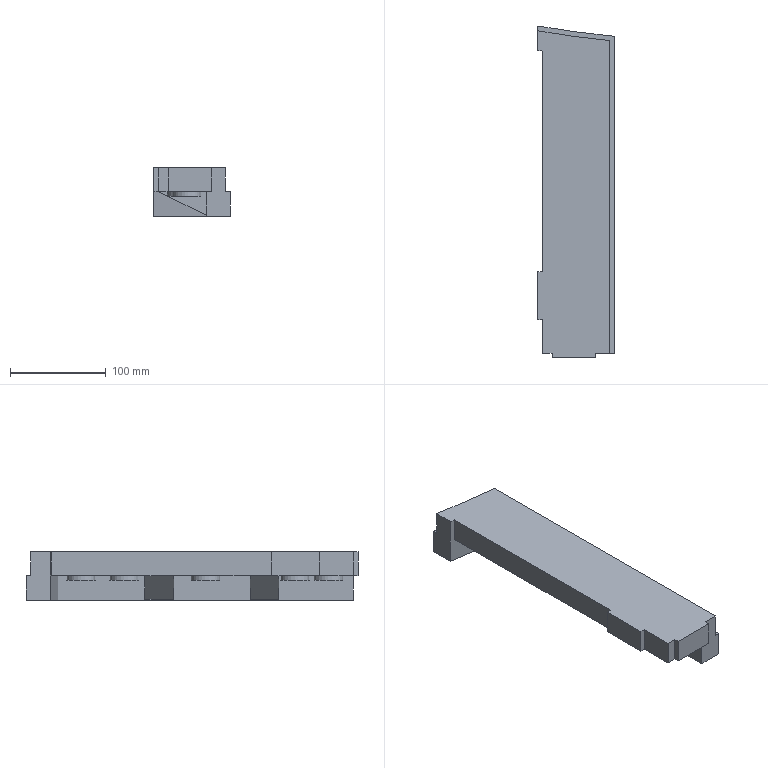Part | NX | features solid 2 | 1 solid | 39 faces | box 80 x 346.995 x 51 mm | volume 901163 mm3 | plane 31 | cylinder 5 | spline 3 | commonest cylinder face diameters 30 x5
STEP:
#1=CARTESIAN_POINT('',(-400.,-480.,45.));
#2=VERTEX_POINT('',#1);
#3=CARTESIAN_POINT('',(-400.,-249.179,45.));
#4=VERTEX_POINT('',#3);
#5=CARTESIAN_POINT('',(-400.,-330.218,45.));
#6=DIRECTION('',(0.,1.,0.));
#7=VECTOR('',#6,1000.);
#8=LINE('',#5,#7);
#9=EDGE_CURVE('',#2,#4,#8,.T.);
#10=ORIENTED_EDGE('',*,*,#9,.T.);
#11=CARTESIAN_POINT('',(-400.,-249.179,20.));
#12=VERTEX_POINT('',#11);
#13=CARTESIAN_POINT('',(-400.,-249.179,45.));
#14=DIRECTION('',(0.,0.,-1.));
#15=VECTOR('',#14,1000.);
#16=LINE('',#13,#15);
#17=EDGE_CURVE('',#4,#12,#16,.T.);
#18=ORIENTED_EDGE('',*,*,#17,.T.);
#19=CARTESIAN_POINT('',(-400.,-347.246,20.));
#20=VERTEX_POINT('',#19);
#21=CARTESIAN_POINT('',(-400.,-330.218,20.));
#22=DIRECTION('',(0.,1.,0.));
#23=VECTOR('',#22,1000.);
#24=LINE('',#21,#23);
#25=EDGE_CURVE('',#20,#12,#24,.T.);
#26=ORIENTED_EDGE('',*,*,#25,.F.);
#27=CARTESIAN_POINT('',(-400.,-377.246,20.));
#28=VERTEX_POINT('',#27);
#29=CARTESIAN_POINT('',(-400.,-347.246,20.));
#30=DIRECTION('',(0.,-1.,0.));
#31=VECTOR('',#30,1000.);
#32=LINE('',#29,#31);
#33=EDGE_CURVE('',#20,#28,#32,.T.);
#34=ORIENTED_EDGE('',*,*,#33,.T.);
#35=CARTESIAN_POINT('',(-400.,-457.246,20.));
#36=VERTEX_POINT('',#35);
#37=CARTESIAN_POINT('',(-400.,-330.218,20.));
#38=DIRECTION('',(0.,1.,0.));
#39=VECTOR('',#38,1000.);
#40=LINE('',#37,#39);
#41=EDGE_CURVE('',#36,#28,#40,.T.);
#42=ORIENTED_EDGE('',*,*,#41,.F.);
#43=CARTESIAN_POINT('',(-400.,-480.,20.));
#44=VERTEX_POINT('',#43);
#45=CARTESIAN_POINT('',(-400.,-457.246,20.));
#46=DIRECTION('',(0.,-1.,0.));
#47=VECTOR('',#46,1000.);
#48=LINE('',#45,#47);
#49=EDGE_CURVE('',#36,#44,#48,.T.);
#50=ORIENTED_EDGE('',*,*,#49,.T.);
#51=CARTESIAN_POINT('',(-400.,-480.,20.));
#52=DIRECTION('',(0.,0.,-1.));
#53=VECTOR('',#52,1000.);
#54=LINE('',#51,#53);
#55=EDGE_CURVE('',#44,#2,#54,.F.);
#56=ORIENTED_EDGE('',*,*,#55,.T.);
#57=EDGE_LOOP('',(#10,#18,#26,#34,#42,#50,#56));
#58=FACE_BOUND('',#57,.T.);
#59=CARTESIAN_POINT('',(-400.,-330.218,45.));
#60=DIRECTION('',(-1.,0.,0.));
#61=DIRECTION('',(0.,0.,1.));
#62=AXIS2_PLACEMENT_3D('',#59,#60,#61);
#63=PLANE('',#62);
#64=ADVANCED_FACE('',(#58),#63,.T.);
#65=CARTESIAN_POINT('',(-350.,-256.193,20.));
#66=VERTEX_POINT('',#65);
#67=CARTESIAN_POINT('',(-350.,-347.246,20.));
#68=VERTEX_POINT('',#67);
#69=CARTESIAN_POINT('',(-350.,-401.561,20.));
#70=DIRECTION('',(0.,1.,0.));
#71=VECTOR('',#70,1000.);
#72=LINE('',#69,#71);
#73=EDGE_CURVE('',#66,#68,#72,.F.);
#74=ORIENTED_EDGE('',*,*,#73,.F.);
#75=CARTESIAN_POINT('',(-350.,-256.193,-6.));
#76=VERTEX_POINT('',#75);
#77=CARTESIAN_POINT('',(-350.,-256.193,45.));
#78=DIRECTION('',(0.,0.,-1.));
#79=VECTOR('',#78,1000.);
#80=LINE('',#77,#79);
#81=EDGE_CURVE('',#66,#76,#80,.T.);
#82=ORIENTED_EDGE('',*,*,#81,.T.);
#83=CARTESIAN_POINT('',(-350.,-565.,-6.));
#84=VERTEX_POINT('',#83);
#85=CARTESIAN_POINT('',(-350.,-1052.635,-6.));
#86=DIRECTION('',(0.,-1.,0.));
#87=VECTOR('',#86,1000.);
#88=LINE('',#85,#87);
#89=EDGE_CURVE('',#84,#76,#88,.F.);
#90=ORIENTED_EDGE('',*,*,#89,.F.);
#91=CARTESIAN_POINT('',(-350.,-565.,20.));
#92=VERTEX_POINT('',#91);
#93=CARTESIAN_POINT('',(-350.,-565.,25.));
#94=DIRECTION('',(0.,0.,1.));
#95=VECTOR('',#94,1000.);
#96=LINE('',#93,#95);
#97=EDGE_CURVE('',#92,#84,#96,.F.);
#98=ORIENTED_EDGE('',*,*,#97,.F.);
#99=CARTESIAN_POINT('',(-350.,-487.246,20.));
#100=VERTEX_POINT('',#99);
#101=CARTESIAN_POINT('',(-350.,-401.561,20.));
#102=DIRECTION('',(0.,1.,0.));
#103=VECTOR('',#102,1000.);
#104=LINE('',#101,#103);
#105=EDGE_CURVE('',#100,#92,#104,.F.);
#106=ORIENTED_EDGE('',*,*,#105,.F.);
#107=CARTESIAN_POINT('',(-350.,-487.246,-5.));
#108=VERTEX_POINT('',#107);
#109=CARTESIAN_POINT('',(-350.,-487.246,20.));
#110=DIRECTION('',(0.,0.,-1.));
#111=VECTOR('',#110,1000.);
#112=LINE('',#109,#111);
#113=EDGE_CURVE('',#100,#108,#112,.T.);
#114=ORIENTED_EDGE('',*,*,#113,.T.);
#115=CARTESIAN_POINT('',(-350.,-457.246,-5.));
#116=VERTEX_POINT('',#115);
#117=CARTESIAN_POINT('',(-350.,-457.246,-5.));
#118=DIRECTION('',(0.,1.,0.));
#119=VECTOR('',#118,1000.);
#120=LINE('',#117,#119);
#121=EDGE_CURVE('',#116,#108,#120,.F.);
#122=ORIENTED_EDGE('',*,*,#121,.F.);
#123=CARTESIAN_POINT('',(-350.,-457.246,20.));
#124=VERTEX_POINT('',#123);
#125=CARTESIAN_POINT('',(-350.,-457.246,20.));
#126=DIRECTION('',(0.,0.,-1.));
#127=VECTOR('',#126,1000.);
#128=LINE('',#125,#127);
#129=EDGE_CURVE('',#124,#116,#128,.T.);
#130=ORIENTED_EDGE('',*,*,#129,.F.);
#131=CARTESIAN_POINT('',(-350.,-377.246,20.));
#132=VERTEX_POINT('',#131);
#133=CARTESIAN_POINT('',(-350.,-401.561,20.));
#134=DIRECTION('',(0.,1.,0.));
#135=VECTOR('',#134,1000.);
#136=LINE('',#133,#135);
#137=EDGE_CURVE('',#132,#124,#136,.F.);
#138=ORIENTED_EDGE('',*,*,#137,.F.);
#139=CARTESIAN_POINT('',(-350.,-377.246,-5.));
#140=VERTEX_POINT('',#139);
#141=CARTESIAN_POINT('',(-350.,-377.246,20.));
#142=DIRECTION('',(0.,0.,-1.));
#143=VECTOR('',#142,1000.);
#144=LINE('',#141,#143);
#145=EDGE_CURVE('',#132,#140,#144,.T.);
#146=ORIENTED_EDGE('',*,*,#145,.T.);
#147=CARTESIAN_POINT('',(-350.,-347.246,-5.));
#148=VERTEX_POINT('',#147);
#149=CARTESIAN_POINT('',(-350.,-347.246,-5.));
#150=DIRECTION('',(0.,1.,0.));
#151=VECTOR('',#150,1000.);
#152=LINE('',#149,#151);
#153=EDGE_CURVE('',#148,#140,#152,.F.);
#154=ORIENTED_EDGE('',*,*,#153,.F.);
#155=CARTESIAN_POINT('',(-350.,-347.246,20.));
#156=DIRECTION('',(0.,0.,-1.));
#157=VECTOR('',#156,1000.);
#158=LINE('',#155,#157);
#159=EDGE_CURVE('',#68,#148,#158,.T.);
#160=ORIENTED_EDGE('',*,*,#159,.F.);
#161=EDGE_LOOP('',(#74,#82,#90,#98,#106,#114,#122,#130,#138,#146,#154,#160));
#162=FACE_BOUND('',#161,.T.);
#163=CARTESIAN_POINT('',(-350.,-560.,25.));
#164=DIRECTION('',(-1.,0.,0.));
#165=DIRECTION('',(0.,0.,1.));
#166=AXIS2_PLACEMENT_3D('',#163,#164,#165);
#167=PLANE('',#166);
#168=ADVANCED_FACE('',(#162),#167,.T.);
#169=CARTESIAN_POINT('',(-390.,-565.,20.));
#170=VERTEX_POINT('',#169);
#171=CARTESIAN_POINT('',(-400.,-565.,20.));
#172=VERTEX_POINT('',#171);
#173=CARTESIAN_POINT('',(-53.05,-565.,20.));
#174=DIRECTION('',(-1.,0.,0.));
#175=VECTOR('',#174,1000.);
#176=LINE('',#173,#175);
#177=EDGE_CURVE('',#170,#172,#176,.T.);
#178=ORIENTED_EDGE('',*,*,#177,.F.);
#179=CARTESIAN_POINT('',(-390.,-565.,45.));
#180=VERTEX_POINT('',#179);
#181=CARTESIAN_POINT('',(-390.,-565.,25.));
#182=DIRECTION('',(0.,0.,-1.));
#183=VECTOR('',#182,1000.);
#184=LINE('',#181,#183);
#185=EDGE_CURVE('',#170,#180,#184,.F.);
#186=ORIENTED_EDGE('',*,*,#185,.T.);
#187=CARTESIAN_POINT('',(-400.,-565.,45.));
#188=VERTEX_POINT('',#187);
#189=CARTESIAN_POINT('',(-582.311,-565.,45.));
#190=DIRECTION('',(1.,0.,0.));
#191=VECTOR('',#190,1000.);
#192=LINE('',#189,#191);
#193=EDGE_CURVE('',#180,#188,#192,.F.);
#194=ORIENTED_EDGE('',*,*,#193,.T.);
#195=CARTESIAN_POINT('',(-400.,-565.,25.));
#196=DIRECTION('',(0.,0.,-1.));
#197=VECTOR('',#196,1000.);
#198=LINE('',#195,#197);
#199=EDGE_CURVE('',#172,#188,#198,.F.);
#200=ORIENTED_EDGE('',*,*,#199,.F.);
#201=EDGE_LOOP('',(#178,#186,#194,#200));
#202=FACE_BOUND('',#201,.T.);
#203=CARTESIAN_POINT('',(-325.,-565.,25.));
#204=DIRECTION('',(0.,-1.,0.));
#205=DIRECTION('',(0.,0.,-1.));
#206=AXIS2_PLACEMENT_3D('',#203,#204,#205);
#207=PLANE('',#206);
#208=ADVANCED_FACE('',(#202),#207,.T.);
#209=ORIENTED_EDGE('',*,*,#25,.T.);
#210=CARTESIAN_POINT('',(-405.,-248.354,20.));
#211=CARTESIAN_POINT('',(-398.879,-249.375,20.));
#212=CARTESIAN_POINT('',(-378.346,-252.669,20.));
#213=CARTESIAN_POINT('',(-351.447,-256.141,20.));
#214=CARTESIAN_POINT('',(-331.018,-258.325,20.));
#215=CARTESIAN_POINT('',(-325.,-258.957,20.));
#216=B_SPLINE_CURVE_WITH_KNOTS('',3,(#210,#211,#212,#213,#214,#215),.UNSPECIFIED.,.F.,.F.,(4,1,1,4),(0.,0.231,0.7722,1.),.UNSPECIFIED.);
#217=EDGE_CURVE('',#12,#66,#216,.T.);
#218=ORIENTED_EDGE('',*,*,#217,.T.);
#219=ORIENTED_EDGE('',*,*,#73,.T.);
#220=CARTESIAN_POINT('',(-350.,-347.246,20.));
#221=DIRECTION('',(-1.,0.,0.));
#222=VECTOR('',#221,1000.);
#223=LINE('',#220,#222);
#224=EDGE_CURVE('',#68,#20,#223,.T.);
#225=ORIENTED_EDGE('',*,*,#224,.T.);
#226=EDGE_LOOP('',(#209,#218,#219,#225));
#227=FACE_BOUND('',#226,.T.);
#228=CARTESIAN_POINT('',(-390.611,-325.558,20.));
#229=VERTEX_POINT('',#228);
#230=CARTESIAN_POINT('',(-375.611,-325.558,20.));
#231=DIRECTION('',(0.,0.,-1.));
#232=DIRECTION('',(-1.,0.,0.));
#233=AXIS2_PLACEMENT_3D('',#230,#231,#232);
#234=CIRCLE('',#233,15.);
#235=EDGE_CURVE('',#229,#229,#234,.T.);
#236=ORIENTED_EDGE('',*,*,#235,.F.);
#237=EDGE_LOOP('',(#236));
#238=FACE_BOUND('',#237,.T.);
#239=CARTESIAN_POINT('',(-385.611,-280.558,20.));
#240=VERTEX_POINT('',#239);
#241=CARTESIAN_POINT('',(-370.611,-280.558,20.));
#242=DIRECTION('',(0.,0.,-1.));
#243=DIRECTION('',(-1.,0.,0.));
#244=AXIS2_PLACEMENT_3D('',#241,#242,#243);
#245=CIRCLE('',#244,15.);
#246=EDGE_CURVE('',#240,#240,#245,.T.);
#247=ORIENTED_EDGE('',*,*,#246,.F.);
#248=EDGE_LOOP('',(#247));
#249=FACE_BOUND('',#248,.T.);
#250=CARTESIAN_POINT('',(-53.05,-401.561,20.));
#251=DIRECTION('',(0.,0.,-1.));
#252=DIRECTION('',(-1.,0.,0.));
#253=AXIS2_PLACEMENT_3D('',#250,#251,#252);
#254=PLANE('',#253);
#255=ADVANCED_FACE('',(#227,#238,#249),#254,.T.);
#256=CARTESIAN_POINT('',(-390.611,-410.558,20.));
#257=VERTEX_POINT('',#256);
#258=CARTESIAN_POINT('',(-375.611,-410.558,20.));
#259=DIRECTION('',(0.,0.,-1.));
#260=DIRECTION('',(-1.,0.,0.));
#261=AXIS2_PLACEMENT_3D('',#258,#259,#260);
#262=CIRCLE('',#261,15.);
#263=EDGE_CURVE('',#257,#257,#262,.T.);
#264=ORIENTED_EDGE('',*,*,#263,.F.);
#265=EDGE_LOOP('',(#264));
#266=FACE_BOUND('',#265,.T.);
#267=ORIENTED_EDGE('',*,*,#137,.T.);
#268=CARTESIAN_POINT('',(-350.,-457.246,20.));
#269=DIRECTION('',(-1.,0.,0.));
#270=VECTOR('',#269,1000.);
#271=LINE('',#268,#270);
#272=EDGE_CURVE('',#124,#36,#271,.T.);
#273=ORIENTED_EDGE('',*,*,#272,.T.);
#274=ORIENTED_EDGE('',*,*,#41,.T.);
#275=CARTESIAN_POINT('',(-350.,-377.246,20.));
#276=DIRECTION('',(-1.,0.,0.));
#277=VECTOR('',#276,1000.);
#278=LINE('',#275,#277);
#279=EDGE_CURVE('',#132,#28,#278,.T.);
#280=ORIENTED_EDGE('',*,*,#279,.F.);
#281=EDGE_LOOP('',(#267,#273,#274,#280));
#282=FACE_BOUND('',#281,.T.);
#283=CARTESIAN_POINT('',(-53.05,-401.561,20.));
#284=DIRECTION('',(0.,0.,-1.));
#285=DIRECTION('',(-1.,0.,0.));
#286=AXIS2_PLACEMENT_3D('',#283,#284,#285);
#287=PLANE('',#286);
#288=ADVANCED_FACE('',(#266,#282),#287,.T.);
#289=CARTESIAN_POINT('',(-390.611,-503.935,20.));
#290=VERTEX_POINT('',#289);
#291=CARTESIAN_POINT('',(-375.611,-503.935,20.));
#292=DIRECTION('',(0.,0.,-1.));
#293=DIRECTION('',(-1.,0.,0.));
#294=AXIS2_PLACEMENT_3D('',#291,#292,#293);
#295=CIRCLE('',#294,15.);
#296=EDGE_CURVE('',#290,#290,#295,.T.);
#297=ORIENTED_EDGE('',*,*,#296,.F.);
#298=EDGE_LOOP('',(#297));
#299=FACE_BOUND('',#298,.T.);
#300=CARTESIAN_POINT('',(-400.,-530.,20.));
#301=VERTEX_POINT('',#300);
#302=CARTESIAN_POINT('',(-400.,-330.218,20.));
#303=DIRECTION('',(0.,1.,0.));
#304=VECTOR('',#303,1000.);
#305=LINE('',#302,#304);
#306=EDGE_CURVE('',#172,#301,#305,.T.);
#307=ORIENTED_EDGE('',*,*,#306,.T.);
#308=CARTESIAN_POINT('',(-405.,-530.,20.));
#309=VERTEX_POINT('',#308);
#310=CARTESIAN_POINT('',(-400.,-530.,20.));
#311=DIRECTION('',(-1.,0.,0.));
#312=VECTOR('',#311,1000.);
#313=LINE('',#310,#312);
#314=EDGE_CURVE('',#301,#309,#313,.T.);
#315=ORIENTED_EDGE('',*,*,#314,.T.);
#316=CARTESIAN_POINT('',(-405.,-480.,20.));
#317=VERTEX_POINT('',#316);
#318=CARTESIAN_POINT('',(-405.,-530.,20.));
#319=DIRECTION('',(0.,1.,0.));
#320=VECTOR('',#319,1000.);
#321=LINE('',#318,#320);
#322=EDGE_CURVE('',#309,#317,#321,.T.);
#323=ORIENTED_EDGE('',*,*,#322,.T.);
#324=CARTESIAN_POINT('',(-400.,-480.,20.));
#325=DIRECTION('',(1.,0.,0.));
#326=VECTOR('',#325,1000.);
#327=LINE('',#324,#326);
#328=EDGE_CURVE('',#44,#317,#327,.F.);
#329=ORIENTED_EDGE('',*,*,#328,.F.);
#330=CARTESIAN_POINT('',(-400.,-487.246,20.));
#331=VERTEX_POINT('',#330);
#332=CARTESIAN_POINT('',(-400.,-457.246,20.));
#333=DIRECTION('',(0.,-1.,0.));
#334=VECTOR('',#333,1000.);
#335=LINE('',#332,#334);
#336=EDGE_CURVE('',#44,#331,#335,.T.);
#337=ORIENTED_EDGE('',*,*,#336,.T.);
#338=CARTESIAN_POINT('',(-350.,-487.246,20.));
#339=DIRECTION('',(-1.,0.,0.));
#340=VECTOR('',#339,1000.);
#341=LINE('',#338,#340);
#342=EDGE_CURVE('',#100,#331,#341,.T.);
#343=ORIENTED_EDGE('',*,*,#342,.F.);
#344=ORIENTED_EDGE('',*,*,#105,.T.);
#345=CARTESIAN_POINT('',(-345.,-565.,20.));
#346=VERTEX_POINT('',#345);
#347=CARTESIAN_POINT('',(-53.05,-565.,20.));
#348=DIRECTION('',(-1.,0.,0.));
#349=VECTOR('',#348,1000.);
#350=LINE('',#347,#349);
#351=EDGE_CURVE('',#346,#92,#350,.T.);
#352=ORIENTED_EDGE('',*,*,#351,.F.);
#353=CARTESIAN_POINT('',(-345.,-570.,20.));
#354=VERTEX_POINT('',#353);
#355=CARTESIAN_POINT('',(-345.,-565.,20.));
#356=DIRECTION('',(0.,1.,0.));
#357=VECTOR('',#356,1000.);
#358=LINE('',#355,#357);
#359=EDGE_CURVE('',#354,#346,#358,.T.);
#360=ORIENTED_EDGE('',*,*,#359,.F.);
#361=CARTESIAN_POINT('',(-390.,-570.,20.));
#362=VERTEX_POINT('',#361);
#363=CARTESIAN_POINT('',(-53.05,-570.,20.));
#364=DIRECTION('',(-1.,0.,0.));
#365=VECTOR('',#364,1000.);
#366=LINE('',#363,#365);
#367=EDGE_CURVE('',#354,#362,#366,.T.);
#368=ORIENTED_EDGE('',*,*,#367,.T.);
#369=CARTESIAN_POINT('',(-390.,-565.,20.));
#370=DIRECTION('',(0.,1.,0.));
#371=VECTOR('',#370,1000.);
#372=LINE('',#369,#371);
#373=EDGE_CURVE('',#362,#170,#372,.T.);
#374=ORIENTED_EDGE('',*,*,#373,.T.);
#375=ORIENTED_EDGE('',*,*,#177,.T.);
#376=EDGE_LOOP('',(#307,#315,#323,#329,#337,#343,#344,#352,#360,#368,#374,#375));
#377=FACE_BOUND('',#376,.T.);
#378=CARTESIAN_POINT('',(-385.611,-538.935,20.));
#379=VERTEX_POINT('',#378);
#380=CARTESIAN_POINT('',(-370.611,-538.935,20.));
#381=DIRECTION('',(0.,0.,-1.));
#382=DIRECTION('',(-1.,0.,0.));
#383=AXIS2_PLACEMENT_3D('',#380,#381,#382);
#384=CIRCLE('',#383,15.);
#385=EDGE_CURVE('',#379,#379,#384,.T.);
#386=ORIENTED_EDGE('',*,*,#385,.F.);
#387=EDGE_LOOP('',(#386));
#388=FACE_BOUND('',#387,.T.);
#389=CARTESIAN_POINT('',(-53.05,-401.561,20.));
#390=DIRECTION('',(0.,0.,-1.));
#391=DIRECTION('',(-1.,0.,0.));
#392=AXIS2_PLACEMENT_3D('',#389,#390,#391);
#393=PLANE('',#392);
#394=ADVANCED_FACE('',(#299,#377,#388),#393,.T.);
#395=CARTESIAN_POINT('',(-330.,-565.,45.));
#396=VERTEX_POINT('',#395);
#397=CARTESIAN_POINT('',(-345.,-565.,45.));
#398=VERTEX_POINT('',#397);
#399=CARTESIAN_POINT('',(-582.311,-565.,45.));
#400=DIRECTION('',(1.,0.,0.));
#401=VECTOR('',#400,1000.);
#402=LINE('',#399,#401);
#403=EDGE_CURVE('',#396,#398,#402,.F.);
#404=ORIENTED_EDGE('',*,*,#403,.T.);
#405=CARTESIAN_POINT('',(-345.,-565.,25.));
#406=DIRECTION('',(0.,0.,1.));
#407=VECTOR('',#406,1000.);
#408=LINE('',#405,#407);
#409=EDGE_CURVE('',#398,#346,#408,.F.);
#410=ORIENTED_EDGE('',*,*,#409,.T.);
#411=ORIENTED_EDGE('',*,*,#351,.T.);
#412=ORIENTED_EDGE('',*,*,#97,.T.);
#413=CARTESIAN_POINT('',(-325.,-565.,-6.));
#414=VERTEX_POINT('',#413);
#415=CARTESIAN_POINT('',(-582.311,-565.,-6.));
#416=DIRECTION('',(1.,0.,0.));
#417=VECTOR('',#416,1000.);
#418=LINE('',#415,#417);
#419=EDGE_CURVE('',#414,#84,#418,.F.);
#420=ORIENTED_EDGE('',*,*,#419,.F.);
#421=CARTESIAN_POINT('',(-325.,-565.,20.));
#422=VERTEX_POINT('',#421);
#423=CARTESIAN_POINT('',(-325.,-565.,25.));
#424=DIRECTION('',(0.,0.,1.));
#425=VECTOR('',#424,1000.);
#426=LINE('',#423,#425);
#427=EDGE_CURVE('',#422,#414,#426,.F.);
#428=ORIENTED_EDGE('',*,*,#427,.F.);
#429=CARTESIAN_POINT('',(-330.,-565.,20.));
#430=VERTEX_POINT('',#429);
#431=CARTESIAN_POINT('',(-325.,-565.,20.));
#432=DIRECTION('',(-1.,0.,0.));
#433=VECTOR('',#432,1000.);
#434=LINE('',#431,#433);
#435=EDGE_CURVE('',#422,#430,#434,.T.);
#436=ORIENTED_EDGE('',*,*,#435,.T.);
#437=CARTESIAN_POINT('',(-330.,-565.,45.));
#438=DIRECTION('',(0.,0.,1.));
#439=VECTOR('',#438,1000.);
#440=LINE('',#437,#439);
#441=EDGE_CURVE('',#396,#430,#440,.F.);
#442=ORIENTED_EDGE('',*,*,#441,.F.);
#443=EDGE_LOOP('',(#404,#410,#411,#412,#420,#428,#436,#442));
#444=FACE_BOUND('',#443,.T.);
#445=CARTESIAN_POINT('',(-325.,-565.,25.));
#446=DIRECTION('',(0.,-1.,0.));
#447=DIRECTION('',(0.,0.,-1.));
#448=AXIS2_PLACEMENT_3D('',#445,#446,#447);
#449=PLANE('',#448);
#450=ADVANCED_FACE('',(#444),#449,.T.);
#451=CARTESIAN_POINT('',(-405.,-248.354,45.));
#452=VERTEX_POINT('',#451);
#453=CARTESIAN_POINT('',(-405.,-248.354,45.));
#454=CARTESIAN_POINT('',(-398.879,-249.375,45.));
#455=CARTESIAN_POINT('',(-378.346,-252.669,45.));
#456=CARTESIAN_POINT('',(-351.447,-256.141,45.));
#457=CARTESIAN_POINT('',(-331.018,-258.325,45.));
#458=CARTESIAN_POINT('',(-325.,-258.957,45.));
#459=B_SPLINE_CURVE_WITH_KNOTS('',3,(#453,#454,#455,#456,#457,#458),.UNSPECIFIED.,.F.,.F.,(4,1,1,4),(0.,0.231,0.7722,1.),.UNSPECIFIED.);
#460=EDGE_CURVE('',#452,#4,#459,.T.);
#461=ORIENTED_EDGE('',*,*,#460,.T.);
#462=ORIENTED_EDGE('',*,*,#9,.F.);
#463=CARTESIAN_POINT('',(-405.,-480.,45.));
#464=VERTEX_POINT('',#463);
#465=CARTESIAN_POINT('',(-400.,-480.,45.));
#466=DIRECTION('',(1.,0.,0.));
#467=VECTOR('',#466,1000.);
#468=LINE('',#465,#467);
#469=EDGE_CURVE('',#2,#464,#468,.F.);
#470=ORIENTED_EDGE('',*,*,#469,.T.);
#471=CARTESIAN_POINT('',(-405.,-530.,45.));
#472=VERTEX_POINT('',#471);
#473=CARTESIAN_POINT('',(-405.,-530.,45.));
#474=DIRECTION('',(0.,1.,0.));
#475=VECTOR('',#474,1000.);
#476=LINE('',#473,#475);
#477=EDGE_CURVE('',#472,#464,#476,.T.);
#478=ORIENTED_EDGE('',*,*,#477,.F.);
#479=CARTESIAN_POINT('',(-400.,-530.,45.));
#480=VERTEX_POINT('',#479);
#481=CARTESIAN_POINT('',(-400.,-530.,45.));
#482=DIRECTION('',(-1.,0.,0.));
#483=VECTOR('',#482,1000.);
#484=LINE('',#481,#483);
#485=EDGE_CURVE('',#480,#472,#484,.T.);
#486=ORIENTED_EDGE('',*,*,#485,.F.);
#487=CARTESIAN_POINT('',(-400.,-330.218,45.));
#488=DIRECTION('',(0.,1.,0.));
#489=VECTOR('',#488,1000.);
#490=LINE('',#487,#489);
#491=EDGE_CURVE('',#188,#480,#490,.T.);
#492=ORIENTED_EDGE('',*,*,#491,.F.);
#493=ORIENTED_EDGE('',*,*,#193,.F.);
#494=CARTESIAN_POINT('',(-390.,-570.,45.));
#495=VERTEX_POINT('',#494);
#496=CARTESIAN_POINT('',(-390.,-565.,45.));
#497=DIRECTION('',(0.,1.,0.));
#498=VECTOR('',#497,1000.);
#499=LINE('',#496,#498);
#500=EDGE_CURVE('',#495,#180,#499,.T.);
#501=ORIENTED_EDGE('',*,*,#500,.F.);
#502=CARTESIAN_POINT('',(-345.,-570.,45.));
#503=VERTEX_POINT('',#502);
#504=CARTESIAN_POINT('',(-582.311,-570.,45.));
#505=DIRECTION('',(1.,0.,0.));
#506=VECTOR('',#505,1000.);
#507=LINE('',#504,#506);
#508=EDGE_CURVE('',#503,#495,#507,.F.);
#509=ORIENTED_EDGE('',*,*,#508,.F.);
#510=CARTESIAN_POINT('',(-345.,-565.,45.));
#511=DIRECTION('',(0.,1.,0.));
#512=VECTOR('',#511,1000.);
#513=LINE('',#510,#512);
#514=EDGE_CURVE('',#503,#398,#513,.T.);
#515=ORIENTED_EDGE('',*,*,#514,.T.);
#516=ORIENTED_EDGE('',*,*,#403,.F.);
#517=CARTESIAN_POINT('',(-330.,-238.313,45.));
#518=VERTEX_POINT('',#517);
#519=CARTESIAN_POINT('',(-330.,-348.688,45.));
#520=DIRECTION('',(0.,1.,0.));
#521=VECTOR('',#520,1000.);
#522=LINE('',#519,#521);
#523=EDGE_CURVE('',#396,#518,#522,.T.);
#524=ORIENTED_EDGE('',*,*,#523,.T.);
#525=CARTESIAN_POINT('',(-405.,-228.076,45.));
#526=VERTEX_POINT('',#525);
#527=CARTESIAN_POINT('',(-330.,-238.313,45.));
#528=CARTESIAN_POINT('',(-333.46,-237.942,45.));
#529=CARTESIAN_POINT('',(-340.216,-237.198,45.));
#530=CARTESIAN_POINT('',(-349.855,-236.075,45.));
#531=CARTESIAN_POINT('',(-357.487,-235.132,45.));
#532=CARTESIAN_POINT('',(-362.599,-234.471,45.));
#533=CARTESIAN_POINT('',(-365.481,-234.089,45.));
#534=CARTESIAN_POINT('',(-367.55,-233.811,45.));
#535=CARTESIAN_POINT('',(-369.827,-233.5,45.));
#536=CARTESIAN_POINT('',(-372.814,-233.084,45.));
#537=CARTESIAN_POINT('',(-378.12,-232.329,45.));
#538=CARTESIAN_POINT('',(-388.899,-230.724,45.));
#539=CARTESIAN_POINT('',(-398.474,-229.18,45.));
#540=CARTESIAN_POINT('',(-405.,-228.076,45.));
#541=B_SPLINE_CURVE_WITH_KNOTS('',3,(#527,#528,#529,#530,#531,#532,#533,#534,#535,#536,#537,#538,#539,#540),.UNSPECIFIED.,.F.,.F.,(4,1,1,1,1,1,1,1,1,1,1,4),(0.,0.125,0.25,0.375,0.4375,0.4688,0.5,0.5312,0.5625,0.625,0.75,1.),.UNSPECIFIED.);
#542=EDGE_CURVE('',#518,#526,#541,.T.);
#543=ORIENTED_EDGE('',*,*,#542,.T.);
#544=CARTESIAN_POINT('',(-405.,-248.354,45.));
#545=DIRECTION('',(0.,1.,0.));
#546=VECTOR('',#545,1000.);
#547=LINE('',#544,#546);
#548=EDGE_CURVE('',#452,#526,#547,.T.);
#549=ORIENTED_EDGE('',*,*,#548,.F.);
#550=EDGE_LOOP('',(#461,#462,#470,#478,#486,#492,#493,#501,#509,#515,#516,#524,#543,#549));
#551=FACE_BOUND('',#550,.T.);
#552=CARTESIAN_POINT('',(-582.311,-1052.635,45.));
#553=DIRECTION('',(0.,0.,1.));
#554=DIRECTION('',(1.,0.,0.));
#555=AXIS2_PLACEMENT_3D('',#552,#553,#554);
#556=PLANE('',#555);
#557=ADVANCED_FACE('',(#551),#556,.T.);
#558=CARTESIAN_POINT('',(-325.,-233.817,20.));
#559=VERTEX_POINT('',#558);
#560=CARTESIAN_POINT('',(-325.,-401.561,20.));
#561=DIRECTION('',(0.,1.,0.));
#562=VECTOR('',#561,1000.);
#563=LINE('',#560,#562);
#564=EDGE_CURVE('',#559,#422,#563,.F.);
#565=ORIENTED_EDGE('',*,*,#564,.T.);
#566=ORIENTED_EDGE('',*,*,#427,.T.);
#567=CARTESIAN_POINT('',(-325.,-233.817,-6.));
#568=VERTEX_POINT('',#567);
#569=CARTESIAN_POINT('',(-325.,-1052.635,-6.));
#570=DIRECTION('',(0.,1.,0.));
#571=VECTOR('',#570,1000.);
#572=LINE('',#569,#571);
#573=EDGE_CURVE('',#414,#568,#572,.T.);
#574=ORIENTED_EDGE('',*,*,#573,.T.);
#575=CARTESIAN_POINT('',(-325.,-233.817,45.));
#576=DIRECTION('',(0.,0.,-1.));
#577=VECTOR('',#576,1000.);
#578=LINE('',#575,#577);
#579=EDGE_CURVE('',#559,#568,#578,.T.);
#580=ORIENTED_EDGE('',*,*,#579,.F.);
#581=EDGE_LOOP('',(#565,#566,#574,#580));
#582=FACE_BOUND('',#581,.T.);
#583=CARTESIAN_POINT('',(-325.,-560.,0.));
#584=DIRECTION('',(1.,0.,0.));
#585=DIRECTION('',(0.,0.,-1.));
#586=AXIS2_PLACEMENT_3D('',#583,#584,#585);
#587=PLANE('',#586);
#588=ADVANCED_FACE('',(#582),#587,.T.);
#589=CARTESIAN_POINT('',(-330.,-238.313,20.));
#590=VERTEX_POINT('',#589);
#591=CARTESIAN_POINT('',(-330.,-238.313,32.5));
#592=DIRECTION('',(0.,0.,1.));
#593=VECTOR('',#592,1000.);
#594=LINE('',#591,#593);
#595=EDGE_CURVE('',#590,#518,#594,.T.);
#596=ORIENTED_EDGE('',*,*,#595,.T.);
#597=ORIENTED_EDGE('',*,*,#523,.F.);
#598=ORIENTED_EDGE('',*,*,#441,.T.);
#599=CARTESIAN_POINT('',(-330.,-348.688,20.));
#600=DIRECTION('',(0.,1.,0.));
#601=VECTOR('',#600,1000.);
#602=LINE('',#599,#601);
#603=EDGE_CURVE('',#430,#590,#602,.T.);
#604=ORIENTED_EDGE('',*,*,#603,.T.);
#605=EDGE_LOOP('',(#596,#597,#598,#604));
#606=FACE_BOUND('',#605,.T.);
#607=CARTESIAN_POINT('',(-330.,-348.688,45.));
#608=DIRECTION('',(-1.,0.,0.));
#609=DIRECTION('',(0.,0.,1.));
#610=AXIS2_PLACEMENT_3D('',#607,#608,#609);
#611=PLANE('',#610);
#612=ADVANCED_FACE('',(#606),#611,.F.);
#613=ORIENTED_EDGE('',*,*,#435,.F.);
#614=ORIENTED_EDGE('',*,*,#564,.F.);
#615=CARTESIAN_POINT('',(-405.,-223.005,20.));
#616=VERTEX_POINT('',#615);
#617=CARTESIAN_POINT('',(-405.,-223.005,20.));
#618=CARTESIAN_POINT('',(-398.446,-224.117,20.));
#619=CARTESIAN_POINT('',(-378.189,-227.424,20.));
#620=CARTESIAN_POINT('',(-351.502,-230.963,20.));
#621=CARTESIAN_POINT('',(-331.353,-233.145,20.));
#622=CARTESIAN_POINT('',(-325.,-233.817,20.));
#623=B_SPLINE_CURVE_WITH_KNOTS('',3,(#617,#618,#619,#620,#621,#622),.UNSPECIFIED.,.F.,.F.,(4,1,1,4),(0.,0.247,0.7626,1.),.UNSPECIFIED.);
#624=EDGE_CURVE('',#559,#616,#623,.F.);
#625=ORIENTED_EDGE('',*,*,#624,.T.);
#626=CARTESIAN_POINT('',(-405.,-228.076,20.));
#627=VERTEX_POINT('',#626);
#628=CARTESIAN_POINT('',(-405.,-248.354,20.));
#629=DIRECTION('',(0.,-1.,0.));
#630=VECTOR('',#629,1000.);
#631=LINE('',#628,#630);
#632=EDGE_CURVE('',#616,#627,#631,.T.);
#633=ORIENTED_EDGE('',*,*,#632,.T.);
#634=CARTESIAN_POINT('',(-405.,-228.076,20.));
#635=CARTESIAN_POINT('',(-392.569,-230.178,20.));
#636=CARTESIAN_POINT('',(-367.6,-234.04,20.));
#637=CARTESIAN_POINT('',(-342.52,-236.97,20.));
#638=CARTESIAN_POINT('',(-330.,-238.313,20.));
#639=B_SPLINE_CURVE_WITH_KNOTS('',3,(#634,#635,#636,#637,#638),.UNSPECIFIED.,.F.,.F.,(4,1,4),(0.01047,0.4774,0.9444),.UNSPECIFIED.);
#640=EDGE_CURVE('',#627,#590,#639,.T.);
#641=ORIENTED_EDGE('',*,*,#640,.T.);
#642=ORIENTED_EDGE('',*,*,#603,.F.);
#643=EDGE_LOOP('',(#613,#614,#625,#633,#641,#642));
#644=FACE_BOUND('',#643,.T.);
#645=CARTESIAN_POINT('',(-53.05,-401.561,20.));
#646=DIRECTION('',(0.,0.,1.));
#647=DIRECTION('',(1.,0.,0.));
#648=AXIS2_PLACEMENT_3D('',#645,#646,#647);
#649=PLANE('',#648);
#650=ADVANCED_FACE('',(#644),#649,.T.);
#651=ORIENTED_EDGE('',*,*,#89,.T.);
#652=CARTESIAN_POINT('',(-405.,-248.354,-6.));
#653=VERTEX_POINT('',#652);
#654=CARTESIAN_POINT('',(-405.,-248.354,-6.));
#655=CARTESIAN_POINT('',(-398.879,-249.375,-6.));
#656=CARTESIAN_POINT('',(-378.346,-252.669,-6.));
#657=CARTESIAN_POINT('',(-351.447,-256.141,-6.));
#658=CARTESIAN_POINT('',(-331.018,-258.325,-6.));
#659=CARTESIAN_POINT('',(-325.,-258.957,-6.));
#660=B_SPLINE_CURVE_WITH_KNOTS('',3,(#654,#655,#656,#657,#658,#659),.UNSPECIFIED.,.F.,.F.,(4,1,1,4),(0.,0.231,0.7722,1.),.UNSPECIFIED.);
#661=EDGE_CURVE('',#653,#76,#660,.T.);
#662=ORIENTED_EDGE('',*,*,#661,.F.);
#663=CARTESIAN_POINT('',(-405.,-223.005,-6.));
#664=VERTEX_POINT('',#663);
#665=CARTESIAN_POINT('',(-405.,-1052.635,-6.));
#666=DIRECTION('',(0.,1.,0.));
#667=VECTOR('',#666,1000.);
#668=LINE('',#665,#667);
#669=EDGE_CURVE('',#653,#664,#668,.T.);
#670=ORIENTED_EDGE('',*,*,#669,.T.);
#671=CARTESIAN_POINT('',(-405.,-223.005,-6.));
#672=CARTESIAN_POINT('',(-398.446,-224.117,-6.));
#673=CARTESIAN_POINT('',(-378.189,-227.424,-6.));
#674=CARTESIAN_POINT('',(-351.502,-230.963,-6.));
#675=CARTESIAN_POINT('',(-331.353,-233.145,-6.));
#676=CARTESIAN_POINT('',(-325.,-233.817,-6.));
#677=B_SPLINE_CURVE_WITH_KNOTS('',3,(#671,#672,#673,#674,#675,#676),.UNSPECIFIED.,.F.,.F.,(4,1,1,4),(0.,0.247,0.7626,1.),.UNSPECIFIED.);
#678=EDGE_CURVE('',#664,#568,#677,.T.);
#679=ORIENTED_EDGE('',*,*,#678,.T.);
#680=ORIENTED_EDGE('',*,*,#573,.F.);
#681=ORIENTED_EDGE('',*,*,#419,.T.);
#682=EDGE_LOOP('',(#651,#662,#670,#679,#680,#681));
#683=FACE_BOUND('',#682,.T.);
#684=CARTESIAN_POINT('',(-582.311,-1052.635,-6.));
#685=DIRECTION('',(0.,0.,1.));
#686=DIRECTION('',(1.,0.,0.));
#687=AXIS2_PLACEMENT_3D('',#684,#685,#686);
#688=PLANE('',#687);
#689=ADVANCED_FACE('',(#683),#688,.F.);
#690=ORIENTED_EDGE('',*,*,#669,.F.);
#691=CARTESIAN_POINT('',(-405.,-248.354,45.));
#692=DIRECTION('',(0.,0.,-1.));
#693=VECTOR('',#692,1000.);
#694=LINE('',#691,#693);
#695=EDGE_CURVE('',#452,#653,#694,.T.);
#696=ORIENTED_EDGE('',*,*,#695,.F.);
#697=ORIENTED_EDGE('',*,*,#548,.T.);
#698=CARTESIAN_POINT('',(-405.,-228.076,37.));
#699=DIRECTION('',(0.,0.,1.));
#700=VECTOR('',#699,1000.);
#701=LINE('',#698,#700);
#702=EDGE_CURVE('',#627,#526,#701,.T.);
#703=ORIENTED_EDGE('',*,*,#702,.F.);
#704=ORIENTED_EDGE('',*,*,#632,.F.);
#705=CARTESIAN_POINT('',(-405.,-223.005,45.));
#706=DIRECTION('',(0.,0.,-1.));
#707=VECTOR('',#706,1000.);
#708=LINE('',#705,#707);
#709=EDGE_CURVE('',#616,#664,#708,.T.);
#710=ORIENTED_EDGE('',*,*,#709,.T.);
#711=EDGE_LOOP('',(#690,#696,#697,#703,#704,#710));
#712=FACE_BOUND('',#711,.T.);
#713=CARTESIAN_POINT('',(-405.,-560.,0.));
#714=DIRECTION('',(1.,0.,0.));
#715=DIRECTION('',(0.,0.,-1.));
#716=AXIS2_PLACEMENT_3D('',#713,#714,#715);
#717=PLANE('',#716);
#718=ADVANCED_FACE('',(#712),#717,.F.);
#719=CARTESIAN_POINT('',(-400.,-530.,20.));
#720=DIRECTION('',(0.,0.,1.));
#721=VECTOR('',#720,1000.);
#722=LINE('',#719,#721);
#723=EDGE_CURVE('',#301,#480,#722,.T.);
#724=ORIENTED_EDGE('',*,*,#723,.F.);
#725=ORIENTED_EDGE('',*,*,#306,.F.);
#726=ORIENTED_EDGE('',*,*,#199,.T.);
#727=ORIENTED_EDGE('',*,*,#491,.T.);
#728=EDGE_LOOP('',(#724,#725,#726,#727));
#729=FACE_BOUND('',#728,.T.);
#730=CARTESIAN_POINT('',(-400.,-330.218,45.));
#731=DIRECTION('',(-1.,0.,0.));
#732=DIRECTION('',(0.,0.,1.));
#733=AXIS2_PLACEMENT_3D('',#730,#731,#732);
#734=PLANE('',#733);
#735=ADVANCED_FACE('',(#729),#734,.T.);
#736=CARTESIAN_POINT('',(-360.611,-325.558,15.));
#737=VERTEX_POINT('',#736);
#738=CARTESIAN_POINT('',(-375.611,-325.558,15.));
#739=DIRECTION('',(0.,0.,1.));
#740=DIRECTION('',(1.,0.,0.));
#741=AXIS2_PLACEMENT_3D('',#738,#739,#740);
#742=CIRCLE('',#741,15.);
#743=EDGE_CURVE('',#737,#737,#742,.T.);
#744=ORIENTED_EDGE('',*,*,#743,.T.);
#745=EDGE_LOOP('',(#744));
#746=FACE_BOUND('',#745,.T.);
#747=ORIENTED_EDGE('',*,*,#235,.T.);
#748=EDGE_LOOP('',(#747));
#749=FACE_BOUND('',#748,.T.);
#750=CARTESIAN_POINT('',(-375.611,-325.558,25.));
#751=DIRECTION('',(0.,0.,-1.));
#752=DIRECTION('',(-1.,0.,0.));
#753=AXIS2_PLACEMENT_3D('',#750,#751,#752);
#754=CYLINDRICAL_SURFACE('',#753,15.);
#755=ADVANCED_FACE('',(#746,#749),#754,.T.);
#756=ORIENTED_EDGE('',*,*,#743,.F.);
#757=EDGE_LOOP('',(#756));
#758=FACE_BOUND('',#757,.T.);
#759=CARTESIAN_POINT('',(-375.611,-325.558,15.));
#760=DIRECTION('',(0.,0.,1.));
#761=DIRECTION('',(1.,0.,0.));
#762=AXIS2_PLACEMENT_3D('',#759,#760,#761);
#763=PLANE('',#762);
#764=ADVANCED_FACE('',(#758),#763,.F.);
#765=ORIENTED_EDGE('',*,*,#159,.T.);
#766=CARTESIAN_POINT('',(-360.,-347.246,0.));
#767=DIRECTION('',(-0.8944,0.,0.4472));
#768=VECTOR('',#767,1000.);
#769=LINE('',#766,#768);
#770=EDGE_CURVE('',#148,#20,#769,.T.);
#771=ORIENTED_EDGE('',*,*,#770,.T.);
#772=ORIENTED_EDGE('',*,*,#224,.F.);
#773=EDGE_LOOP('',(#765,#771,#772));
#774=FACE_BOUND('',#773,.T.);
#775=CARTESIAN_POINT('',(-350.,-347.246,20.));
#776=DIRECTION('',(0.,1.,0.));
#777=DIRECTION('',(-1.,0.,0.));
#778=AXIS2_PLACEMENT_3D('',#775,#776,#777);
#779=PLANE('',#778);
#780=ADVANCED_FACE('',(#774),#779,.T.);
#781=ORIENTED_EDGE('',*,*,#279,.T.);
#782=CARTESIAN_POINT('',(-360.,-377.246,0.));
#783=DIRECTION('',(-0.8944,0.,0.4472));
#784=VECTOR('',#783,1000.);
#785=LINE('',#782,#784);
#786=EDGE_CURVE('',#28,#140,#785,.F.);
#787=ORIENTED_EDGE('',*,*,#786,.T.);
#788=ORIENTED_EDGE('',*,*,#145,.F.);
#789=EDGE_LOOP('',(#781,#787,#788));
#790=FACE_BOUND('',#789,.T.);
#791=CARTESIAN_POINT('',(-350.,-377.246,20.));
#792=DIRECTION('',(0.,1.,0.));
#793=DIRECTION('',(-1.,0.,0.));
#794=AXIS2_PLACEMENT_3D('',#791,#792,#793);
#795=PLANE('',#794);
#796=ADVANCED_FACE('',(#790),#795,.F.);
#797=ORIENTED_EDGE('',*,*,#770,.F.);
#798=ORIENTED_EDGE('',*,*,#153,.T.);
#799=ORIENTED_EDGE('',*,*,#786,.F.);
#800=ORIENTED_EDGE('',*,*,#33,.F.);
#801=EDGE_LOOP('',(#797,#798,#799,#800));
#802=FACE_BOUND('',#801,.T.);
#803=CARTESIAN_POINT('',(-400.,-347.246,20.));
#804=DIRECTION('',(-0.4472,0.,-0.8944));
#805=DIRECTION('',(-0.8944,0.,0.4472));
#806=AXIS2_PLACEMENT_3D('',#803,#804,#805);
#807=PLANE('',#806);
#808=ADVANCED_FACE('',(#802),#807,.T.);
#809=CARTESIAN_POINT('',(-360.611,-410.558,15.));
#810=VERTEX_POINT('',#809);
#811=CARTESIAN_POINT('',(-375.611,-410.558,15.));
#812=DIRECTION('',(0.,0.,1.));
#813=DIRECTION('',(1.,0.,0.));
#814=AXIS2_PLACEMENT_3D('',#811,#812,#813);
#815=CIRCLE('',#814,15.);
#816=EDGE_CURVE('',#810,#810,#815,.T.);
#817=ORIENTED_EDGE('',*,*,#816,.T.);
#818=EDGE_LOOP('',(#817));
#819=FACE_BOUND('',#818,.T.);
#820=ORIENTED_EDGE('',*,*,#263,.T.);
#821=EDGE_LOOP('',(#820));
#822=FACE_BOUND('',#821,.T.);
#823=CARTESIAN_POINT('',(-375.611,-410.558,25.));
#824=DIRECTION('',(0.,0.,-1.));
#825=DIRECTION('',(-1.,0.,0.));
#826=AXIS2_PLACEMENT_3D('',#823,#824,#825);
#827=CYLINDRICAL_SURFACE('',#826,15.);
#828=ADVANCED_FACE('',(#819,#822),#827,.T.);
#829=ORIENTED_EDGE('',*,*,#816,.F.);
#830=EDGE_LOOP('',(#829));
#831=FACE_BOUND('',#830,.T.);
#832=CARTESIAN_POINT('',(-375.611,-410.558,15.));
#833=DIRECTION('',(0.,0.,1.));
#834=DIRECTION('',(1.,0.,0.));
#835=AXIS2_PLACEMENT_3D('',#832,#833,#834);
#836=PLANE('',#835);
#837=ADVANCED_FACE('',(#831),#836,.F.);
#838=CARTESIAN_POINT('',(-360.611,-503.935,15.));
#839=VERTEX_POINT('',#838);
#840=CARTESIAN_POINT('',(-375.611,-503.935,15.));
#841=DIRECTION('',(0.,0.,-1.));
#842=DIRECTION('',(1.,0.,0.));
#843=AXIS2_PLACEMENT_3D('',#840,#841,#842);
#844=CIRCLE('',#843,15.);
#845=EDGE_CURVE('',#839,#839,#844,.T.);
#846=ORIENTED_EDGE('',*,*,#845,.F.);
#847=EDGE_LOOP('',(#846));
#848=FACE_BOUND('',#847,.T.);
#849=ORIENTED_EDGE('',*,*,#296,.T.);
#850=EDGE_LOOP('',(#849));
#851=FACE_BOUND('',#850,.T.);
#852=CARTESIAN_POINT('',(-375.611,-503.935,25.));
#853=DIRECTION('',(0.,0.,-1.));
#854=DIRECTION('',(-1.,0.,0.));
#855=AXIS2_PLACEMENT_3D('',#852,#853,#854);
#856=CYLINDRICAL_SURFACE('',#855,15.);
#857=ADVANCED_FACE('',(#848,#851),#856,.T.);
#858=ORIENTED_EDGE('',*,*,#845,.T.);
#859=EDGE_LOOP('',(#858));
#860=FACE_BOUND('',#859,.T.);
#861=CARTESIAN_POINT('',(-375.611,-503.935,15.));
#862=DIRECTION('',(0.,0.,1.));
#863=DIRECTION('',(1.,0.,0.));
#864=AXIS2_PLACEMENT_3D('',#861,#862,#863);
#865=PLANE('',#864);
#866=ADVANCED_FACE('',(#860),#865,.F.);
#867=CARTESIAN_POINT('',(-355.611,-538.935,15.));
#868=VERTEX_POINT('',#867);
#869=CARTESIAN_POINT('',(-370.611,-538.935,15.));
#870=DIRECTION('',(0.,0.,-1.));
#871=DIRECTION('',(1.,0.,0.));
#872=AXIS2_PLACEMENT_3D('',#869,#870,#871);
#873=CIRCLE('',#872,15.);
#874=EDGE_CURVE('',#868,#868,#873,.T.);
#875=ORIENTED_EDGE('',*,*,#874,.F.);
#876=EDGE_LOOP('',(#875));
#877=FACE_BOUND('',#876,.T.);
#878=ORIENTED_EDGE('',*,*,#385,.T.);
#879=EDGE_LOOP('',(#878));
#880=FACE_BOUND('',#879,.T.);
#881=CARTESIAN_POINT('',(-370.611,-538.935,25.));
#882=DIRECTION('',(0.,0.,-1.));
#883=DIRECTION('',(-1.,0.,0.));
#884=AXIS2_PLACEMENT_3D('',#881,#882,#883);
#885=CYLINDRICAL_SURFACE('',#884,15.);
#886=ADVANCED_FACE('',(#877,#880),#885,.T.);
#887=ORIENTED_EDGE('',*,*,#874,.T.);
#888=EDGE_LOOP('',(#887));
#889=FACE_BOUND('',#888,.T.);
#890=CARTESIAN_POINT('',(-370.611,-538.935,15.));
#891=DIRECTION('',(0.,0.,1.));
#892=DIRECTION('',(1.,0.,0.));
#893=AXIS2_PLACEMENT_3D('',#890,#891,#892);
#894=PLANE('',#893);
#895=ADVANCED_FACE('',(#889),#894,.F.);
#896=ORIENTED_EDGE('',*,*,#129,.T.);
#897=CARTESIAN_POINT('',(-360.,-457.246,0.));
#898=DIRECTION('',(-0.8944,0.,0.4472));
#899=VECTOR('',#898,1000.);
#900=LINE('',#897,#899);
#901=EDGE_CURVE('',#116,#36,#900,.T.);
#902=ORIENTED_EDGE('',*,*,#901,.T.);
#903=ORIENTED_EDGE('',*,*,#272,.F.);
#904=EDGE_LOOP('',(#896,#902,#903));
#905=FACE_BOUND('',#904,.T.);
#906=CARTESIAN_POINT('',(-350.,-457.246,20.));
#907=DIRECTION('',(0.,1.,0.));
#908=DIRECTION('',(-1.,0.,0.));
#909=AXIS2_PLACEMENT_3D('',#906,#907,#908);
#910=PLANE('',#909);
#911=ADVANCED_FACE('',(#905),#910,.T.);
#912=ORIENTED_EDGE('',*,*,#342,.T.);
#913=CARTESIAN_POINT('',(-360.,-487.246,0.));
#914=DIRECTION('',(-0.8944,0.,0.4472));
#915=VECTOR('',#914,1000.);
#916=LINE('',#913,#915);
#917=EDGE_CURVE('',#331,#108,#916,.F.);
#918=ORIENTED_EDGE('',*,*,#917,.T.);
#919=ORIENTED_EDGE('',*,*,#113,.F.);
#920=EDGE_LOOP('',(#912,#918,#919));
#921=FACE_BOUND('',#920,.T.);
#922=CARTESIAN_POINT('',(-350.,-487.246,20.));
#923=DIRECTION('',(0.,1.,0.));
#924=DIRECTION('',(-1.,0.,0.));
#925=AXIS2_PLACEMENT_3D('',#922,#923,#924);
#926=PLANE('',#925);
#927=ADVANCED_FACE('',(#921),#926,.F.);
#928=ORIENTED_EDGE('',*,*,#901,.F.);
#929=ORIENTED_EDGE('',*,*,#121,.T.);
#930=ORIENTED_EDGE('',*,*,#917,.F.);
#931=ORIENTED_EDGE('',*,*,#336,.F.);
#932=ORIENTED_EDGE('',*,*,#49,.F.);
#933=EDGE_LOOP('',(#928,#929,#930,#931,#932));
#934=FACE_BOUND('',#933,.T.);
#935=CARTESIAN_POINT('',(-400.,-457.246,20.));
#936=DIRECTION('',(-0.4472,0.,-0.8944));
#937=DIRECTION('',(-0.8944,0.,0.4472));
#938=AXIS2_PLACEMENT_3D('',#935,#936,#937);
#939=PLANE('',#938);
#940=ADVANCED_FACE('',(#934),#939,.T.);
#941=CARTESIAN_POINT('',(-355.611,-280.558,15.));
#942=VERTEX_POINT('',#941);
#943=CARTESIAN_POINT('',(-370.611,-280.558,15.));
#944=DIRECTION('',(0.,0.,1.));
#945=DIRECTION('',(1.,0.,0.));
#946=AXIS2_PLACEMENT_3D('',#943,#944,#945);
#947=CIRCLE('',#946,15.);
#948=EDGE_CURVE('',#942,#942,#947,.T.);
#949=ORIENTED_EDGE('',*,*,#948,.T.);
#950=EDGE_LOOP('',(#949));
#951=FACE_BOUND('',#950,.T.);
#952=ORIENTED_EDGE('',*,*,#246,.T.);
#953=EDGE_LOOP('',(#952));
#954=FACE_BOUND('',#953,.T.);
#955=CARTESIAN_POINT('',(-370.611,-280.558,25.));
#956=DIRECTION('',(0.,0.,-1.));
#957=DIRECTION('',(-1.,0.,0.));
#958=AXIS2_PLACEMENT_3D('',#955,#956,#957);
#959=CYLINDRICAL_SURFACE('',#958,15.);
#960=ADVANCED_FACE('',(#951,#954),#959,.T.);
#961=ORIENTED_EDGE('',*,*,#948,.F.);
#962=EDGE_LOOP('',(#961));
#963=FACE_BOUND('',#962,.T.);
#964=CARTESIAN_POINT('',(-370.611,-280.558,15.));
#965=DIRECTION('',(0.,0.,1.));
#966=DIRECTION('',(1.,0.,0.));
#967=AXIS2_PLACEMENT_3D('',#964,#965,#966);
#968=PLANE('',#967);
#969=ADVANCED_FACE('',(#963),#968,.F.);
#970=ORIENTED_EDGE('',*,*,#185,.F.);
#971=ORIENTED_EDGE('',*,*,#373,.F.);
#972=CARTESIAN_POINT('',(-390.,-570.,25.));
#973=DIRECTION('',(0.,0.,-1.));
#974=VECTOR('',#973,1000.);
#975=LINE('',#972,#974);
#976=EDGE_CURVE('',#362,#495,#975,.F.);
#977=ORIENTED_EDGE('',*,*,#976,.T.);
#978=ORIENTED_EDGE('',*,*,#500,.T.);
#979=EDGE_LOOP('',(#970,#971,#977,#978));
#980=FACE_BOUND('',#979,.T.);
#981=CARTESIAN_POINT('',(-390.,-565.,25.));
#982=DIRECTION('',(-1.,0.,0.));
#983=DIRECTION('',(0.,0.,1.));
#984=AXIS2_PLACEMENT_3D('',#981,#982,#983);
#985=PLANE('',#984);
#986=ADVANCED_FACE('',(#980),#985,.T.);
#987=ORIENTED_EDGE('',*,*,#409,.F.);
#988=ORIENTED_EDGE('',*,*,#514,.F.);
#989=CARTESIAN_POINT('',(-345.,-570.,25.));
#990=DIRECTION('',(0.,0.,1.));
#991=VECTOR('',#990,1000.);
#992=LINE('',#989,#991);
#993=EDGE_CURVE('',#503,#354,#992,.F.);
#994=ORIENTED_EDGE('',*,*,#993,.T.);
#995=ORIENTED_EDGE('',*,*,#359,.T.);
#996=EDGE_LOOP('',(#987,#988,#994,#995));
#997=FACE_BOUND('',#996,.T.);
#998=CARTESIAN_POINT('',(-345.,-565.,25.));
#999=DIRECTION('',(1.,0.,0.));
#1000=DIRECTION('',(0.,0.,-1.));
#1001=AXIS2_PLACEMENT_3D('',#998,#999,#1000);
#1002=PLANE('',#1001);
#1003=ADVANCED_FACE('',(#997),#1002,.T.);
#1004=ORIENTED_EDGE('',*,*,#976,.F.);
#1005=ORIENTED_EDGE('',*,*,#367,.F.);
#1006=ORIENTED_EDGE('',*,*,#993,.F.);
#1007=ORIENTED_EDGE('',*,*,#508,.T.);
#1008=EDGE_LOOP('',(#1004,#1005,#1006,#1007));
#1009=FACE_BOUND('',#1008,.T.);
#1010=CARTESIAN_POINT('',(-325.,-570.,25.));
#1011=DIRECTION('',(0.,-1.,0.));
#1012=DIRECTION('',(0.,0.,-1.));
#1013=AXIS2_PLACEMENT_3D('',#1010,#1011,#1012);
#1014=PLANE('',#1013);
#1015=ADVANCED_FACE('',(#1009),#1014,.T.);
#1016=ORIENTED_EDGE('',*,*,#322,.F.);
#1017=CARTESIAN_POINT('',(-405.,-530.,20.));
#1018=DIRECTION('',(0.,0.,1.));
#1019=VECTOR('',#1018,1000.);
#1020=LINE('',#1017,#1019);
#1021=EDGE_CURVE('',#309,#472,#1020,.T.);
#1022=ORIENTED_EDGE('',*,*,#1021,.T.);
#1023=ORIENTED_EDGE('',*,*,#477,.T.);
#1024=CARTESIAN_POINT('',(-405.,-480.,20.));
#1025=DIRECTION('',(0.,0.,-1.));
#1026=VECTOR('',#1025,1000.);
#1027=LINE('',#1024,#1026);
#1028=EDGE_CURVE('',#317,#464,#1027,.F.);
#1029=ORIENTED_EDGE('',*,*,#1028,.F.);
#1030=EDGE_LOOP('',(#1016,#1022,#1023,#1029));
#1031=FACE_BOUND('',#1030,.T.);
#1032=CARTESIAN_POINT('',(-405.,-530.,20.));
#1033=DIRECTION('',(1.,0.,0.));
#1034=DIRECTION('',(0.,0.,1.));
#1035=AXIS2_PLACEMENT_3D('',#1032,#1033,#1034);
#1036=PLANE('',#1035);
#1037=ADVANCED_FACE('',(#1031),#1036,.F.);
#1038=ORIENTED_EDGE('',*,*,#1028,.T.);
#1039=ORIENTED_EDGE('',*,*,#469,.F.);
#1040=ORIENTED_EDGE('',*,*,#55,.F.);
#1041=ORIENTED_EDGE('',*,*,#328,.T.);
#1042=EDGE_LOOP('',(#1038,#1039,#1040,#1041));
#1043=FACE_BOUND('',#1042,.T.);
#1044=CARTESIAN_POINT('',(-400.,-480.,20.));
#1045=DIRECTION('',(0.,-1.,0.));
#1046=DIRECTION('',(0.,0.,-1.));
#1047=AXIS2_PLACEMENT_3D('',#1044,#1045,#1046);
#1048=PLANE('',#1047);
#1049=ADVANCED_FACE('',(#1043),#1048,.F.);
#1050=ORIENTED_EDGE('',*,*,#1021,.F.);
#1051=ORIENTED_EDGE('',*,*,#314,.F.);
#1052=ORIENTED_EDGE('',*,*,#723,.T.);
#1053=ORIENTED_EDGE('',*,*,#485,.T.);
#1054=EDGE_LOOP('',(#1050,#1051,#1052,#1053));
#1055=FACE_BOUND('',#1054,.T.);
#1056=CARTESIAN_POINT('',(-400.,-530.,20.));
#1057=DIRECTION('',(0.,-1.,0.));
#1058=DIRECTION('',(0.,0.,-1.));
#1059=AXIS2_PLACEMENT_3D('',#1056,#1057,#1058);
#1060=PLANE('',#1059);
#1061=ADVANCED_FACE('',(#1055),#1060,.T.);
#1062=ORIENTED_EDGE('',*,*,#595,.F.);
#1063=ORIENTED_EDGE('',*,*,#640,.F.);
#1064=ORIENTED_EDGE('',*,*,#702,.T.);
#1065=ORIENTED_EDGE('',*,*,#542,.F.);
#1066=EDGE_LOOP('',(#1062,#1063,#1064,#1065));
#1067=FACE_BOUND('',#1066,.T.);
#1068=CARTESIAN_POINT('',(-405.,-228.076,20.));
#1069=CARTESIAN_POINT('',(-405.,-228.076,45.));
#1070=CARTESIAN_POINT('',(-392.569,-230.178,20.));
#1071=CARTESIAN_POINT('',(-392.569,-230.178,45.));
#1072=CARTESIAN_POINT('',(-367.6,-234.04,20.));
#1073=CARTESIAN_POINT('',(-367.6,-234.04,45.));
#1074=CARTESIAN_POINT('',(-342.52,-236.97,20.));
#1075=CARTESIAN_POINT('',(-342.52,-236.97,45.));
#1076=CARTESIAN_POINT('',(-330.,-238.313,20.));
#1077=CARTESIAN_POINT('',(-330.,-238.313,45.));
#1078=B_SPLINE_SURFACE_WITH_KNOTS('',3,1,((#1068,#1069),(#1070,#1071),(#1072,#1073),(#1074,#1075),(#1076,#1077)),.SURF_OF_LINEAR_EXTRUSION.,.F.,.F.,.F.,(4,1,4),(2,2),(0.01047,0.4774,0.9444),(0.,1.),.UNSPECIFIED.);
#1079=ADVANCED_FACE('',(#1067),#1078,.F.);
#1080=ORIENTED_EDGE('',*,*,#17,.F.);
#1081=ORIENTED_EDGE('',*,*,#460,.F.);
#1082=ORIENTED_EDGE('',*,*,#695,.T.);
#1083=ORIENTED_EDGE('',*,*,#661,.T.);
#1084=ORIENTED_EDGE('',*,*,#81,.F.);
#1085=ORIENTED_EDGE('',*,*,#217,.F.);
#1086=EDGE_LOOP('',(#1080,#1081,#1082,#1083,#1084,#1085));
#1087=FACE_BOUND('',#1086,.T.);
#1088=CARTESIAN_POINT('',(-405.,-248.354,45.));
#1089=CARTESIAN_POINT('',(-405.,-248.354,-6.));
#1090=CARTESIAN_POINT('',(-386.808,-251.389,45.));
#1091=CARTESIAN_POINT('',(-386.808,-251.389,-6.));
#1092=CARTESIAN_POINT('',(-368.351,-254.016,45.));
#1093=CARTESIAN_POINT('',(-368.351,-254.016,-6.));
#1094=CARTESIAN_POINT('',(-350.,-256.193,45.));
#1095=CARTESIAN_POINT('',(-350.,-256.193,-6.));
#1096=B_SPLINE_SURFACE_WITH_KNOTS('',3,1,((#1088,#1089),(#1090,#1091),(#1092,#1093),(#1094,#1095)),.SURF_OF_LINEAR_EXTRUSION.,.F.,.F.,.F.,(4,4),(2,2),(0.,0.6866),(0.,1.),.PIECEWISE_BEZIER_KNOTS.);
#1097=ADVANCED_FACE('',(#1087),#1096,.F.);
#1098=ORIENTED_EDGE('',*,*,#624,.F.);
#1099=ORIENTED_EDGE('',*,*,#579,.T.);
#1100=ORIENTED_EDGE('',*,*,#678,.F.);
#1101=ORIENTED_EDGE('',*,*,#709,.F.);
#1102=EDGE_LOOP('',(#1098,#1099,#1100,#1101));
#1103=FACE_BOUND('',#1102,.T.);
#1104=CARTESIAN_POINT('',(-405.,-223.005,20.));
#1105=CARTESIAN_POINT('',(-405.,-223.005,-6.));
#1106=CARTESIAN_POINT('',(-391.732,-225.256,20.));
#1107=CARTESIAN_POINT('',(-391.732,-225.256,-6.));
#1108=CARTESIAN_POINT('',(-365.129,-229.363,20.));
#1109=CARTESIAN_POINT('',(-365.129,-229.363,-6.));
#1110=CARTESIAN_POINT('',(-338.383,-232.402,20.));
#1111=CARTESIAN_POINT('',(-338.383,-232.402,-6.));
#1112=CARTESIAN_POINT('',(-325.,-233.817,20.));
#1113=CARTESIAN_POINT('',(-325.,-233.817,-6.));
#1114=B_SPLINE_SURFACE_WITH_KNOTS('',3,1,((#1104,#1105),(#1106,#1107),(#1108,#1109),(#1110,#1111),(#1112,#1113)),.SURF_OF_LINEAR_EXTRUSION.,.F.,.F.,.F.,(4,1,4),(2,2),(0.,0.5,1.),(0.,1.),.UNSPECIFIED.);
#1115=ADVANCED_FACE('',(#1103),#1114,.T.);
#1116=CLOSED_SHELL('',(#64,#168,#208,#255,#288,#394,#450,#557,#588,#612,#650,#689,#718,#735,#755,#764,#780,#796,#808,#828,#837,#857,#866,#886,#895,#911,#927,#940,#960,#969,#986,#1003,#1015,#1037,#1049,#1061,#1079,#1097,#1115));
#1117=MANIFOLD_SOLID_BREP('',#1116);
#1118=(LENGTH_UNIT()NAMED_UNIT(*)SI_UNIT(.MILLI.,.METRE.));
#1119=UNCERTAINTY_MEASURE_WITH_UNIT(LENGTH_MEASURE(0.0508),#1118,'','');
#1120=(NAMED_UNIT(*)PLANE_ANGLE_UNIT()SI_UNIT($,.RADIAN.));
#1121=(NAMED_UNIT(*)SI_UNIT($,.STERADIAN.)SOLID_ANGLE_UNIT());
#1122=(GEOMETRIC_REPRESENTATION_CONTEXT(3)GLOBAL_UNCERTAINTY_ASSIGNED_CONTEXT((#1119))GLOBAL_UNIT_ASSIGNED_CONTEXT((#1118,#1120,#1121))REPRESENTATION_CONTEXT('',''));
#1123=ADVANCED_BREP_SHAPE_REPRESENTATION('',(#1117),#1122);